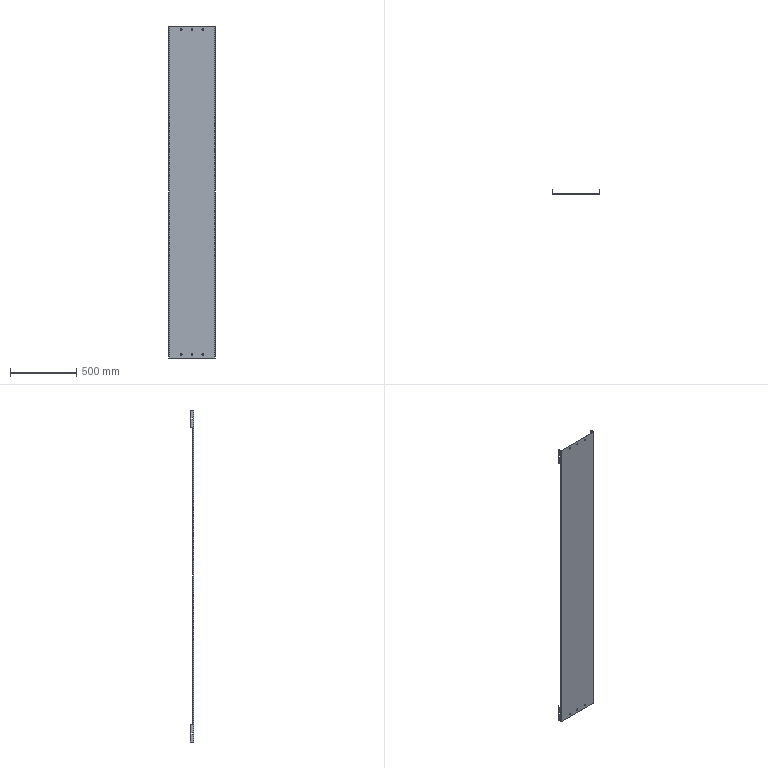Part | SolidWorks | features ICE 3, SMBaseFlange 2, Cut 1, FlatPattern 1, MirrorPattern 1, SheetMetal 1 | 1 solid | 58 faces | box 350 x 30 x 2502 mm | volume 926955 mm3 | plane 42 | cylinder 16 | commonest cylinder face diameters 10.5 x12 2 x2 4 x2